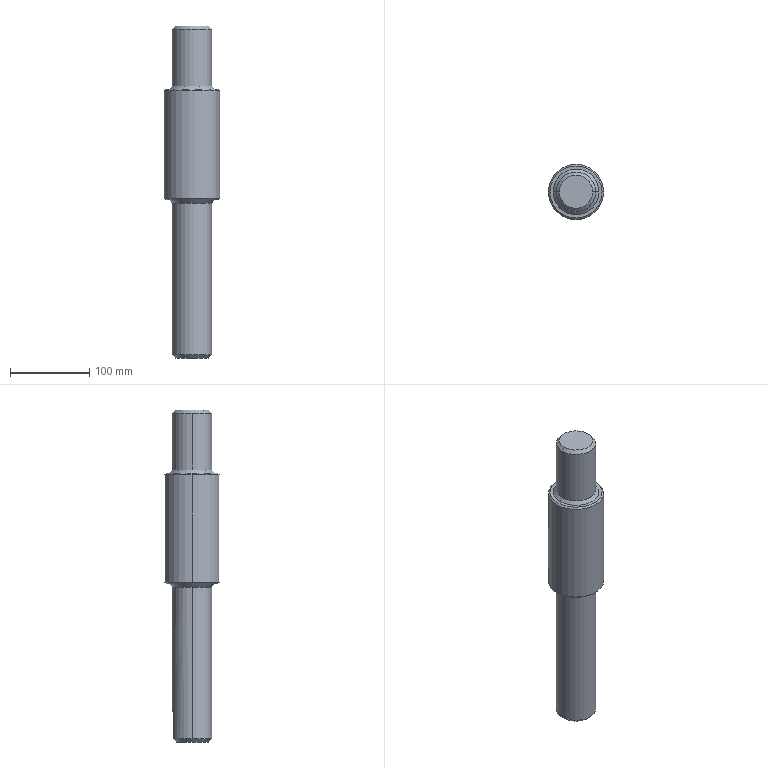Part | SolidWorks | features Chamfer 3, ICE 2, Extrusion 1 | 1 solid | 28 faces | box 70 x 70 x 420 mm | volume 1082180 mm3 | cone 13 | cylinder 8 | plane 7 | commonest cylinder face diameters 50 x4 15 x2 70 x2
STEP:
#1=CARTESIAN_POINT('',(25.,0.,324.));
#2=VERTEX_POINT('',#1);
#3=CARTESIAN_POINT('',(-25.,0.,324.));
#4=VERTEX_POINT('',#3);
#5=CARTESIAN_POINT('',(0.,0.,324.));
#6=DIRECTION('',(0.,0.,1.));
#7=DIRECTION('',(1.,0.,0.));
#8=AXIS2_PLACEMENT_3D('',#5,#6,#7);
#9=CIRCLE('',#8,25.);
#10=EDGE_CURVE('',#2,#4,#9,.T.);
#11=ORIENTED_EDGE('',*,*,#10,.F.);
#12=CARTESIAN_POINT('',(29.,0.,320.));
#13=VERTEX_POINT('',#12);
#14=CARTESIAN_POINT('',(29.,0.,320.));
#15=DIRECTION('',(0.7071,0.,-0.7071));
#16=VECTOR('',#15,1000.);
#17=LINE('',#14,#16);
#18=EDGE_CURVE('',#2,#13,#17,.T.);
#19=ORIENTED_EDGE('',*,*,#18,.T.);
#20=CARTESIAN_POINT('',(-29.,0.,320.));
#21=VERTEX_POINT('',#20);
#22=CARTESIAN_POINT('',(0.,0.,320.));
#23=DIRECTION('',(0.,0.,-1.));
#24=DIRECTION('',(1.,0.,0.));
#25=AXIS2_PLACEMENT_3D('',#22,#23,#24);
#26=CIRCLE('',#25,29.);
#27=EDGE_CURVE('',#21,#13,#26,.T.);
#28=ORIENTED_EDGE('',*,*,#27,.F.);
#29=CARTESIAN_POINT('',(-29.,0.,320.));
#30=DIRECTION('',(-0.7071,0.,-0.7071));
#31=VECTOR('',#30,1000.);
#32=LINE('',#29,#31);
#33=EDGE_CURVE('',#4,#21,#32,.T.);
#34=ORIENTED_EDGE('',*,*,#33,.F.);
#35=EDGE_LOOP('',(#11,#19,#28,#34));
#36=FACE_OUTER_BOUND('',#35,.T.);
#37=CARTESIAN_POINT('',(0.,0.,320.));
#38=DIRECTION('',(0.,0.,-1.));
#39=DIRECTION('',(-1.,0.,0.));
#40=AXIS2_PLACEMENT_3D('',#37,#38,#39);
#41=CONICAL_SURFACE('',#40,29.,0.7854);
#42=ADVANCED_FACE('',(#36),#41,.T.);
#43=CARTESIAN_POINT('',(-25.,0.,176.));
#44=VERTEX_POINT('',#43);
#45=CARTESIAN_POINT('',(25.,0.,176.));
#46=VERTEX_POINT('',#45);
#47=CARTESIAN_POINT('',(0.,0.,176.));
#48=DIRECTION('',(0.,0.,-1.));
#49=DIRECTION('',(1.,0.,0.));
#50=AXIS2_PLACEMENT_3D('',#47,#48,#49);
#51=CIRCLE('',#50,25.);
#52=EDGE_CURVE('',#44,#46,#51,.T.);
#53=ORIENTED_EDGE('',*,*,#52,.F.);
#54=CARTESIAN_POINT('',(-29.,0.,180.));
#55=VERTEX_POINT('',#54);
#56=CARTESIAN_POINT('',(-25.,0.,176.));
#57=DIRECTION('',(-0.7071,0.,0.7071));
#58=VECTOR('',#57,1000.);
#59=LINE('',#56,#58);
#60=EDGE_CURVE('',#44,#55,#59,.T.);
#61=ORIENTED_EDGE('',*,*,#60,.T.);
#62=CARTESIAN_POINT('',(29.,0.,180.));
#63=VERTEX_POINT('',#62);
#64=CARTESIAN_POINT('',(0.,0.,180.));
#65=DIRECTION('',(0.,0.,1.));
#66=DIRECTION('',(1.,0.,0.));
#67=AXIS2_PLACEMENT_3D('',#64,#65,#66);
#68=CIRCLE('',#67,29.);
#69=EDGE_CURVE('',#63,#55,#68,.T.);
#70=ORIENTED_EDGE('',*,*,#69,.F.);
#71=CARTESIAN_POINT('',(25.,0.,176.));
#72=DIRECTION('',(0.7071,0.,0.7071));
#73=VECTOR('',#72,1000.);
#74=LINE('',#71,#73);
#75=EDGE_CURVE('',#46,#63,#74,.T.);
#76=ORIENTED_EDGE('',*,*,#75,.F.);
#77=EDGE_LOOP('',(#53,#61,#70,#76));
#78=FACE_OUTER_BOUND('',#77,.T.);
#79=CARTESIAN_POINT('',(0.,0.,176.));
#80=DIRECTION('',(0.,0.,1.));
#81=DIRECTION('',(1.,0.,0.));
#82=AXIS2_PLACEMENT_3D('',#79,#80,#81);
#83=CONICAL_SURFACE('',#82,25.,0.7854);
#84=ADVANCED_FACE('',(#78),#83,.T.);
#85=CARTESIAN_POINT('',(33.,0.,320.));
#86=VERTEX_POINT('',#85);
#87=CARTESIAN_POINT('',(-33.,0.,320.));
#88=VERTEX_POINT('',#87);
#89=CARTESIAN_POINT('',(0.,0.,320.));
#90=DIRECTION('',(0.,0.,1.));
#91=DIRECTION('',(1.,0.,0.));
#92=AXIS2_PLACEMENT_3D('',#89,#90,#91);
#93=CIRCLE('',#92,33.);
#94=EDGE_CURVE('',#86,#88,#93,.T.);
#95=ORIENTED_EDGE('',*,*,#94,.F.);
#96=CARTESIAN_POINT('',(35.,0.,318.));
#97=VERTEX_POINT('',#96);
#98=CARTESIAN_POINT('',(33.,0.,320.));
#99=DIRECTION('',(0.7071,0.,-0.7071));
#100=VECTOR('',#99,1000.);
#101=LINE('',#98,#100);
#102=EDGE_CURVE('',#86,#97,#101,.T.);
#103=ORIENTED_EDGE('',*,*,#102,.T.);
#104=CARTESIAN_POINT('',(-35.,0.,318.));
#105=VERTEX_POINT('',#104);
#106=CARTESIAN_POINT('',(0.,0.,318.));
#107=DIRECTION('',(0.,0.,-1.));
#108=DIRECTION('',(1.,0.,0.));
#109=AXIS2_PLACEMENT_3D('',#106,#107,#108);
#110=CIRCLE('',#109,35.);
#111=EDGE_CURVE('',#105,#97,#110,.T.);
#112=ORIENTED_EDGE('',*,*,#111,.F.);
#113=CARTESIAN_POINT('',(-33.,0.,320.));
#114=DIRECTION('',(-0.7071,0.,-0.7071));
#115=VECTOR('',#114,1000.);
#116=LINE('',#113,#115);
#117=EDGE_CURVE('',#88,#105,#116,.T.);
#118=ORIENTED_EDGE('',*,*,#117,.F.);
#119=EDGE_LOOP('',(#95,#103,#112,#118));
#120=FACE_OUTER_BOUND('',#119,.T.);
#121=CARTESIAN_POINT('',(0.,0.,320.));
#122=DIRECTION('',(0.,0.,-1.));
#123=DIRECTION('',(-1.,0.,0.));
#124=AXIS2_PLACEMENT_3D('',#121,#122,#123);
#125=CONICAL_SURFACE('',#124,33.,0.7854);
#126=ADVANCED_FACE('',(#120),#125,.T.);
#127=CARTESIAN_POINT('',(-33.,0.,180.));
#128=VERTEX_POINT('',#127);
#129=CARTESIAN_POINT('',(33.,0.,180.));
#130=VERTEX_POINT('',#129);
#131=CARTESIAN_POINT('',(0.,0.,180.));
#132=DIRECTION('',(0.,0.,-1.));
#133=DIRECTION('',(1.,0.,0.));
#134=AXIS2_PLACEMENT_3D('',#131,#132,#133);
#135=CIRCLE('',#134,33.);
#136=EDGE_CURVE('',#128,#130,#135,.T.);
#137=ORIENTED_EDGE('',*,*,#136,.F.);
#138=CARTESIAN_POINT('',(-35.,0.,182.));
#139=VERTEX_POINT('',#138);
#140=CARTESIAN_POINT('',(-35.,0.,182.));
#141=DIRECTION('',(-0.7071,0.,0.7071));
#142=VECTOR('',#141,1000.);
#143=LINE('',#140,#142);
#144=EDGE_CURVE('',#128,#139,#143,.T.);
#145=ORIENTED_EDGE('',*,*,#144,.T.);
#146=CARTESIAN_POINT('',(35.,0.,182.));
#147=VERTEX_POINT('',#146);
#148=CARTESIAN_POINT('',(0.,0.,182.));
#149=DIRECTION('',(0.,0.,1.));
#150=DIRECTION('',(1.,0.,0.));
#151=AXIS2_PLACEMENT_3D('',#148,#149,#150);
#152=CIRCLE('',#151,35.);
#153=EDGE_CURVE('',#147,#139,#152,.T.);
#154=ORIENTED_EDGE('',*,*,#153,.F.);
#155=CARTESIAN_POINT('',(35.,0.,182.));
#156=DIRECTION('',(0.7071,0.,0.7071));
#157=VECTOR('',#156,1000.);
#158=LINE('',#155,#157);
#159=EDGE_CURVE('',#130,#147,#158,.T.);
#160=ORIENTED_EDGE('',*,*,#159,.F.);
#161=EDGE_LOOP('',(#137,#145,#154,#160));
#162=FACE_OUTER_BOUND('',#161,.T.);
#163=CARTESIAN_POINT('',(0.,0.,182.));
#164=DIRECTION('',(0.,0.,1.));
#165=DIRECTION('',(1.,0.,0.));
#166=AXIS2_PLACEMENT_3D('',#163,#164,#165);
#167=CONICAL_SURFACE('',#166,35.,0.7854);
#168=ADVANCED_FACE('',(#162),#167,.T.);
#169=CARTESIAN_POINT('',(-7.5,23.848,-16.));
#170=VERTEX_POINT('',#169);
#171=CARTESIAN_POINT('',(-25.,0.,-16.));
#172=VERTEX_POINT('',#171);
#173=CARTESIAN_POINT('',(0.,0.,-16.));
#174=DIRECTION('',(0.,0.,1.));
#175=DIRECTION('',(1.,0.,0.));
#176=AXIS2_PLACEMENT_3D('',#173,#174,#175);
#177=CIRCLE('',#176,25.);
#178=EDGE_CURVE('',#170,#172,#177,.T.);
#179=ORIENTED_EDGE('',*,*,#178,.T.);
#180=CARTESIAN_POINT('',(-25.,0.,-20.));
#181=DIRECTION('',(0.,0.,1.));
#182=VECTOR('',#181,1000.);
#183=LINE('',#180,#182);
#184=EDGE_CURVE('',#172,#44,#183,.T.);
#185=ORIENTED_EDGE('',*,*,#184,.T.);
#186=ORIENTED_EDGE('',*,*,#52,.T.);
#187=CARTESIAN_POINT('',(25.,0.,-16.));
#188=VERTEX_POINT('',#187);
#189=CARTESIAN_POINT('',(25.,0.,-20.));
#190=DIRECTION('',(0.,0.,1.));
#191=VECTOR('',#190,1000.);
#192=LINE('',#189,#191);
#193=EDGE_CURVE('',#188,#46,#192,.T.);
#194=ORIENTED_EDGE('',*,*,#193,.F.);
#195=CARTESIAN_POINT('',(7.5,23.848,-16.));
#196=VERTEX_POINT('',#195);
#197=CARTESIAN_POINT('',(0.,0.,-16.));
#198=DIRECTION('',(0.,0.,1.));
#199=DIRECTION('',(1.,0.,0.));
#200=AXIS2_PLACEMENT_3D('',#197,#198,#199);
#201=CIRCLE('',#200,25.);
#202=EDGE_CURVE('',#188,#196,#201,.T.);
#203=ORIENTED_EDGE('',*,*,#202,.T.);
#204=CARTESIAN_POINT('',(7.5,23.848,15.));
#205=VERTEX_POINT('',#204);
#206=CARTESIAN_POINT('',(7.5,23.848,-20.));
#207=DIRECTION('',(0.,0.,-1.));
#208=VECTOR('',#207,1000.);
#209=LINE('',#206,#208);
#210=EDGE_CURVE('',#205,#196,#209,.T.);
#211=ORIENTED_EDGE('',*,*,#210,.F.);
#212=CARTESIAN_POINT('',(0.,25.,22.5));
#213=VERTEX_POINT('',#212);
#214=CARTESIAN_POINT('',(0.,25.,22.5));
#215=CARTESIAN_POINT('',(0.492,25.,22.5));
#216=CARTESIAN_POINT('',(0.9918,24.985,22.45));
#217=CARTESIAN_POINT('',(1.955,24.928,22.257));
#218=CARTESIAN_POINT('',(2.424,24.886,22.115));
#219=CARTESIAN_POINT('',(3.107,24.807,21.831));
#220=CARTESIAN_POINT('',(3.331,24.778,21.724));
#221=CARTESIAN_POINT('',(3.762,24.716,21.493));
#222=CARTESIAN_POINT('',(3.971,24.684,21.367));
#223=CARTESIAN_POINT('',(4.375,24.615,21.097));
#224=CARTESIAN_POINT('',(4.571,24.579,20.951));
#225=CARTESIAN_POINT('',(4.948,24.506,20.641));
#226=CARTESIAN_POINT('',(5.131,24.468,20.475));
#227=CARTESIAN_POINT('',(5.65,24.356,19.956));
#228=CARTESIAN_POINT('',(5.958,24.281,19.581));
#229=CARTESIAN_POINT('',(6.501,24.142,18.772));
#230=CARTESIAN_POINT('',(6.736,24.076,18.334));
#231=CARTESIAN_POINT('',(7.112,23.968,17.431));
#232=CARTESIAN_POINT('',(7.255,23.924,16.964));
#233=CARTESIAN_POINT('',(7.401,23.879,16.238));
#234=CARTESIAN_POINT('',(7.438,23.868,15.991));
#235=CARTESIAN_POINT('',(7.488,23.852,15.497));
#236=CARTESIAN_POINT('',(7.5,23.848,15.249));
#237=CARTESIAN_POINT('',(7.5,23.848,15.));
#238=B_SPLINE_CURVE_WITH_KNOTS('',3,(#214,#215,#216,#217,#218,#219,#220,#221,#222,#223,#224,#225,#226,#227,#228,#229,#230,#231,#232,#233,#234,#235,#236,#237),.UNSPECIFIED.,.F.,.F.,(4,2,2,2,2,2,2,2,2,2,2,4),(0.0118,0.01327,0.01474,0.01548,0.01621,0.01695,0.01769,0.01916,0.02063,0.0221,0.02284,0.02358),.UNSPECIFIED.);
#239=EDGE_CURVE('',#213,#205,#238,.T.);
#240=ORIENTED_EDGE('',*,*,#239,.F.);
#241=CARTESIAN_POINT('',(-7.5,23.848,15.));
#242=VERTEX_POINT('',#241);
#243=CARTESIAN_POINT('',(-7.5,23.848,15.));
#244=CARTESIAN_POINT('',(-7.5,23.848,15.499));
#245=CARTESIAN_POINT('',(-7.451,23.864,15.989));
#246=CARTESIAN_POINT('',(-7.306,23.909,16.711));
#247=CARTESIAN_POINT('',(-7.246,23.927,16.949));
#248=CARTESIAN_POINT('',(-7.102,23.97,17.422));
#249=CARTESIAN_POINT('',(-7.018,23.995,17.656));
#250=CARTESIAN_POINT('',(-6.735,24.077,18.336));
#251=CARTESIAN_POINT('',(-6.504,24.141,18.766));
#252=CARTESIAN_POINT('',(-6.096,24.246,19.376));
#253=CARTESIAN_POINT('',(-5.948,24.283,19.574));
#254=CARTESIAN_POINT('',(-5.637,24.357,19.953));
#255=CARTESIAN_POINT('',(-5.473,24.394,20.134));
#256=CARTESIAN_POINT('',(-4.957,24.506,20.649));
#257=CARTESIAN_POINT('',(-4.581,24.58,20.959));
#258=CARTESIAN_POINT('',(-3.761,24.719,21.507));
#259=CARTESIAN_POINT('',(-3.329,24.781,21.738));
#260=CARTESIAN_POINT('',(-2.653,24.86,22.019));
#261=CARTESIAN_POINT('',(-2.423,24.883,22.102));
#262=CARTESIAN_POINT('',(-1.951,24.925,22.246));
#263=CARTESIAN_POINT('',(-1.709,24.943,22.307));
#264=CARTESIAN_POINT('',(-0.9814,24.985,22.452));
#265=CARTESIAN_POINT('',(-0.4926,25.,22.5));
#266=CARTESIAN_POINT('',(0.,25.,22.5));
#267=B_SPLINE_CURVE_WITH_KNOTS('',3,(#243,#244,#245,#246,#247,#248,#249,#250,#251,#252,#253,#254,#255,#256,#257,#258,#259,#260,#261,#262,#263,#264,#265,#266),.UNSPECIFIED.,.F.,.F.,(4,2,2,2,2,2,2,2,2,2,2,4),(0.,0.001474,0.002212,0.002949,0.004423,0.005161,0.005898,0.007372,0.008847,0.009584,0.01032,0.0118),.UNSPECIFIED.);
#268=EDGE_CURVE('',#242,#213,#267,.T.);
#269=ORIENTED_EDGE('',*,*,#268,.F.);
#270=CARTESIAN_POINT('',(-7.5,23.848,-20.));
#271=DIRECTION('',(0.,0.,1.));
#272=VECTOR('',#271,1000.);
#273=LINE('',#270,#272);
#274=EDGE_CURVE('',#170,#242,#273,.T.);
#275=ORIENTED_EDGE('',*,*,#274,.F.);
#276=EDGE_LOOP('',(#179,#185,#186,#194,#203,#211,#240,#269,#275));
#277=FACE_OUTER_BOUND('',#276,.T.);
#278=CARTESIAN_POINT('',(0.,0.,-20.));
#279=DIRECTION('',(0.,0.,1.));
#280=DIRECTION('',(1.,0.,0.));
#281=AXIS2_PLACEMENT_3D('',#278,#279,#280);
#282=CYLINDRICAL_SURFACE('',#281,25.);
#283=ADVANCED_FACE('',(#277),#282,.T.);
#284=CARTESIAN_POINT('',(-21.,0.,-20.));
#285=VERTEX_POINT('',#284);
#286=CARTESIAN_POINT('',(-7.5,19.615,-20.));
#287=VERTEX_POINT('',#286);
#288=CARTESIAN_POINT('',(0.,0.,-20.));
#289=DIRECTION('',(0.,0.,-1.));
#290=DIRECTION('',(1.,0.,0.));
#291=AXIS2_PLACEMENT_3D('',#288,#289,#290);
#292=CIRCLE('',#291,21.);
#293=EDGE_CURVE('',#285,#287,#292,.T.);
#294=ORIENTED_EDGE('',*,*,#293,.F.);
#295=CARTESIAN_POINT('',(-25.,0.,-16.));
#296=DIRECTION('',(-0.7071,0.,0.7071));
#297=VECTOR('',#296,1000.);
#298=LINE('',#295,#297);
#299=EDGE_CURVE('',#285,#172,#298,.T.);
#300=ORIENTED_EDGE('',*,*,#299,.T.);
#301=ORIENTED_EDGE('',*,*,#178,.F.);
#302=CARTESIAN_POINT('',(-7.5,19.615,-20.));
#303=CARTESIAN_POINT('',(-7.5,21.034,-18.675));
#304=CARTESIAN_POINT('',(-7.5,22.444,-17.34));
#305=CARTESIAN_POINT('',(-7.5,23.848,-16.));
#306=B_SPLINE_CURVE_WITH_KNOTS('',3,(#302,#303,#304,#305),.UNSPECIFIED.,.F.,.F.,(4,4),(0.02102,0.02682),.UNSPECIFIED.);
#307=EDGE_CURVE('',#287,#170,#306,.T.);
#308=ORIENTED_EDGE('',*,*,#307,.F.);
#309=EDGE_LOOP('',(#294,#300,#301,#308));
#310=FACE_OUTER_BOUND('',#309,.T.);
#311=CARTESIAN_POINT('',(0.,0.,-16.));
#312=DIRECTION('',(0.,0.,1.));
#313=DIRECTION('',(1.,0.,0.));
#314=AXIS2_PLACEMENT_3D('',#311,#312,#313);
#315=CONICAL_SURFACE('',#314,25.,0.7854);
#316=ADVANCED_FACE('',(#310),#315,.T.);
#317=ORIENTED_EDGE('',*,*,#299,.F.);
#318=CARTESIAN_POINT('',(21.,0.,-20.));
#319=VERTEX_POINT('',#318);
#320=CARTESIAN_POINT('',(0.,0.,-20.));
#321=DIRECTION('',(0.,0.,-1.));
#322=DIRECTION('',(1.,0.,0.));
#323=AXIS2_PLACEMENT_3D('',#320,#321,#322);
#324=CIRCLE('',#323,21.);
#325=EDGE_CURVE('',#319,#285,#324,.T.);
#326=ORIENTED_EDGE('',*,*,#325,.F.);
#327=CARTESIAN_POINT('',(25.,0.,-16.));
#328=DIRECTION('',(0.7071,0.,0.7071));
#329=VECTOR('',#328,1000.);
#330=LINE('',#327,#329);
#331=EDGE_CURVE('',#319,#188,#330,.T.);
#332=ORIENTED_EDGE('',*,*,#331,.T.);
#333=CARTESIAN_POINT('',(0.,0.,-16.));
#334=DIRECTION('',(0.,0.,1.));
#335=DIRECTION('',(1.,0.,0.));
#336=AXIS2_PLACEMENT_3D('',#333,#334,#335);
#337=CIRCLE('',#336,25.);
#338=EDGE_CURVE('',#172,#188,#337,.T.);
#339=ORIENTED_EDGE('',*,*,#338,.F.);
#340=EDGE_LOOP('',(#317,#326,#332,#339));
#341=FACE_OUTER_BOUND('',#340,.T.);
#342=CARTESIAN_POINT('',(0.,0.,-16.));
#343=DIRECTION('',(0.,0.,1.));
#344=DIRECTION('',(1.,0.,0.));
#345=AXIS2_PLACEMENT_3D('',#342,#343,#344);
#346=CONICAL_SURFACE('',#345,25.,0.7854);
#347=ADVANCED_FACE('',(#341),#346,.T.);
#348=CARTESIAN_POINT('',(0.,15.,22.5));
#349=VERTEX_POINT('',#348);
#350=CARTESIAN_POINT('',(7.5,15.,15.));
#351=VERTEX_POINT('',#350);
#352=CARTESIAN_POINT('',(0.,15.,15.));
#353=DIRECTION('',(0.,1.,0.));
#354=DIRECTION('',(0.,0.,1.));
#355=AXIS2_PLACEMENT_3D('',#352,#353,#354);
#356=CIRCLE('',#355,7.5);
#357=EDGE_CURVE('',#349,#351,#356,.T.);
#358=ORIENTED_EDGE('',*,*,#357,.F.);
#359=CARTESIAN_POINT('',(0.,15.,22.5));
#360=DIRECTION('',(0.,1.,0.));
#361=VECTOR('',#360,1000.);
#362=LINE('',#359,#361);
#363=EDGE_CURVE('',#349,#213,#362,.T.);
#364=ORIENTED_EDGE('',*,*,#363,.T.);
#365=ORIENTED_EDGE('',*,*,#239,.T.);
#366=CARTESIAN_POINT('',(7.5,15.,15.));
#367=DIRECTION('',(0.,1.,0.));
#368=VECTOR('',#367,1000.);
#369=LINE('',#366,#368);
#370=EDGE_CURVE('',#351,#205,#369,.T.);
#371=ORIENTED_EDGE('',*,*,#370,.F.);
#372=EDGE_LOOP('',(#358,#364,#365,#371));
#373=FACE_OUTER_BOUND('',#372,.T.);
#374=CARTESIAN_POINT('',(0.,15.,15.));
#375=DIRECTION('',(0.,1.,0.));
#376=DIRECTION('',(0.,0.,1.));
#377=AXIS2_PLACEMENT_3D('',#374,#375,#376);
#378=CYLINDRICAL_SURFACE('',#377,7.5);
#379=ADVANCED_FACE('',(#373),#378,.F.);
#380=ORIENTED_EDGE('',*,*,#111,.T.);
#381=CARTESIAN_POINT('',(35.,0.,320.));
#382=DIRECTION('',(0.,0.,-1.));
#383=VECTOR('',#382,1000.);
#384=LINE('',#381,#383);
#385=EDGE_CURVE('',#97,#147,#384,.T.);
#386=ORIENTED_EDGE('',*,*,#385,.T.);
#387=ORIENTED_EDGE('',*,*,#153,.T.);
#388=CARTESIAN_POINT('',(-35.,0.,320.));
#389=DIRECTION('',(0.,0.,-1.));
#390=VECTOR('',#389,1000.);
#391=LINE('',#388,#390);
#392=EDGE_CURVE('',#105,#139,#391,.T.);
#393=ORIENTED_EDGE('',*,*,#392,.F.);
#394=EDGE_LOOP('',(#380,#386,#387,#393));
#395=FACE_OUTER_BOUND('',#394,.T.);
#396=CARTESIAN_POINT('',(0.,0.,320.));
#397=DIRECTION('',(0.,0.,-1.));
#398=DIRECTION('',(-1.,0.,0.));
#399=AXIS2_PLACEMENT_3D('',#396,#397,#398);
#400=CYLINDRICAL_SURFACE('',#399,35.);
#401=ADVANCED_FACE('',(#395),#400,.T.);
#402=CARTESIAN_POINT('',(21.,0.,400.));
#403=VERTEX_POINT('',#402);
#404=CARTESIAN_POINT('',(-21.,0.,400.));
#405=VERTEX_POINT('',#404);
#406=CARTESIAN_POINT('',(0.,0.,400.));
#407=DIRECTION('',(0.,0.,1.));
#408=DIRECTION('',(1.,0.,0.));
#409=AXIS2_PLACEMENT_3D('',#406,#407,#408);
#410=CIRCLE('',#409,21.);
#411=EDGE_CURVE('',#403,#405,#410,.T.);
#412=ORIENTED_EDGE('',*,*,#411,.F.);
#413=CARTESIAN_POINT('',(25.,0.,396.));
#414=VERTEX_POINT('',#413);
#415=CARTESIAN_POINT('',(21.,0.,400.));
#416=DIRECTION('',(0.7071,0.,-0.7071));
#417=VECTOR('',#416,1000.);
#418=LINE('',#415,#417);
#419=EDGE_CURVE('',#403,#414,#418,.T.);
#420=ORIENTED_EDGE('',*,*,#419,.T.);
#421=CARTESIAN_POINT('',(-25.,0.,396.));
#422=VERTEX_POINT('',#421);
#423=CARTESIAN_POINT('',(0.,0.,396.));
#424=DIRECTION('',(0.,0.,-1.));
#425=DIRECTION('',(1.,0.,0.));
#426=AXIS2_PLACEMENT_3D('',#423,#424,#425);
#427=CIRCLE('',#426,25.);
#428=EDGE_CURVE('',#422,#414,#427,.T.);
#429=ORIENTED_EDGE('',*,*,#428,.F.);
#430=CARTESIAN_POINT('',(-21.,0.,400.));
#431=DIRECTION('',(-0.7071,0.,-0.7071));
#432=VECTOR('',#431,1000.);
#433=LINE('',#430,#432);
#434=EDGE_CURVE('',#405,#422,#433,.T.);
#435=ORIENTED_EDGE('',*,*,#434,.F.);
#436=EDGE_LOOP('',(#412,#420,#429,#435));
#437=FACE_OUTER_BOUND('',#436,.T.);
#438=CARTESIAN_POINT('',(0.,0.,400.));
#439=DIRECTION('',(0.,0.,-1.));
#440=DIRECTION('',(-1.,0.,0.));
#441=AXIS2_PLACEMENT_3D('',#438,#439,#440);
#442=CONICAL_SURFACE('',#441,21.,0.7854);
#443=ADVANCED_FACE('',(#437),#442,.T.);
#444=ORIENTED_EDGE('',*,*,#10,.T.);
#445=CARTESIAN_POINT('',(-25.,0.,-20.));
#446=DIRECTION('',(0.,0.,1.));
#447=VECTOR('',#446,1000.);
#448=LINE('',#445,#447);
#449=EDGE_CURVE('',#4,#422,#448,.T.);
#450=ORIENTED_EDGE('',*,*,#449,.T.);
#451=ORIENTED_EDGE('',*,*,#428,.T.);
#452=CARTESIAN_POINT('',(25.,0.,-20.));
#453=DIRECTION('',(0.,0.,1.));
#454=VECTOR('',#453,1000.);
#455=LINE('',#452,#454);
#456=EDGE_CURVE('',#2,#414,#455,.T.);
#457=ORIENTED_EDGE('',*,*,#456,.F.);
#458=EDGE_LOOP('',(#444,#450,#451,#457));
#459=FACE_OUTER_BOUND('',#458,.T.);
#460=CARTESIAN_POINT('',(0.,0.,-20.));
#461=DIRECTION('',(0.,0.,1.));
#462=DIRECTION('',(1.,0.,0.));
#463=AXIS2_PLACEMENT_3D('',#460,#461,#462);
#464=CYLINDRICAL_SURFACE('',#463,25.);
#465=ADVANCED_FACE('',(#459),#464,.T.);
#466=ORIENTED_EDGE('',*,*,#449,.F.);
#467=CARTESIAN_POINT('',(0.,0.,324.));
#468=DIRECTION('',(0.,0.,1.));
#469=DIRECTION('',(1.,0.,0.));
#470=AXIS2_PLACEMENT_3D('',#467,#468,#469);
#471=CIRCLE('',#470,25.);
#472=EDGE_CURVE('',#4,#2,#471,.T.);
#473=ORIENTED_EDGE('',*,*,#472,.T.);
#474=ORIENTED_EDGE('',*,*,#456,.T.);
#475=CARTESIAN_POINT('',(0.,0.,396.));
#476=DIRECTION('',(0.,0.,-1.));
#477=DIRECTION('',(1.,0.,0.));
#478=AXIS2_PLACEMENT_3D('',#475,#476,#477);
#479=CIRCLE('',#478,25.);
#480=EDGE_CURVE('',#414,#422,#479,.T.);
#481=ORIENTED_EDGE('',*,*,#480,.T.);
#482=EDGE_LOOP('',(#466,#473,#474,#481));
#483=FACE_OUTER_BOUND('',#482,.T.);
#484=CARTESIAN_POINT('',(0.,0.,-20.));
#485=DIRECTION('',(0.,0.,1.));
#486=DIRECTION('',(1.,0.,0.));
#487=AXIS2_PLACEMENT_3D('',#484,#485,#486);
#488=CYLINDRICAL_SURFACE('',#487,25.);
#489=ADVANCED_FACE('',(#483),#488,.T.);
#490=CARTESIAN_POINT('',(0.,0.,400.));
#491=DIRECTION('',(0.,0.,1.));
#492=DIRECTION('',(1.,0.,0.));
#493=AXIS2_PLACEMENT_3D('',#490,#491,#492);
#494=CIRCLE('',#493,21.);
#495=EDGE_CURVE('',#405,#403,#494,.T.);
#496=ORIENTED_EDGE('',*,*,#495,.T.);
#497=ORIENTED_EDGE('',*,*,#411,.T.);
#498=EDGE_LOOP('',(#496,#497));
#499=FACE_OUTER_BOUND('',#498,.T.);
#500=CARTESIAN_POINT('',(0.,0.,400.));
#501=DIRECTION('',(0.,0.,1.));
#502=DIRECTION('',(1.,0.,0.));
#503=AXIS2_PLACEMENT_3D('',#500,#501,#502);
#504=PLANE('',#503);
#505=ADVANCED_FACE('',(#499),#504,.T.);
#506=ORIENTED_EDGE('',*,*,#419,.F.);
#507=ORIENTED_EDGE('',*,*,#495,.F.);
#508=ORIENTED_EDGE('',*,*,#434,.T.);
#509=ORIENTED_EDGE('',*,*,#480,.F.);
#510=EDGE_LOOP('',(#506,#507,#508,#509));
#511=FACE_OUTER_BOUND('',#510,.T.);
#512=CARTESIAN_POINT('',(0.,0.,400.));
#513=DIRECTION('',(0.,0.,-1.));
#514=DIRECTION('',(-1.,0.,0.));
#515=AXIS2_PLACEMENT_3D('',#512,#513,#514);
#516=CONICAL_SURFACE('',#515,21.,0.7854);
#517=ADVANCED_FACE('',(#511),#516,.T.);
#518=ORIENTED_EDGE('',*,*,#385,.F.);
#519=CARTESIAN_POINT('',(0.,0.,318.));
#520=DIRECTION('',(0.,0.,-1.));
#521=DIRECTION('',(1.,0.,0.));
#522=AXIS2_PLACEMENT_3D('',#519,#520,#521);
#523=CIRCLE('',#522,35.);
#524=EDGE_CURVE('',#97,#105,#523,.T.);
#525=ORIENTED_EDGE('',*,*,#524,.T.);
#526=ORIENTED_EDGE('',*,*,#392,.T.);
#527=CARTESIAN_POINT('',(0.,0.,182.));
#528=DIRECTION('',(0.,0.,1.));
#529=DIRECTION('',(1.,0.,0.));
#530=AXIS2_PLACEMENT_3D('',#527,#528,#529);
#531=CIRCLE('',#530,35.);
#532=EDGE_CURVE('',#139,#147,#531,.T.);
#533=ORIENTED_EDGE('',*,*,#532,.T.);
#534=EDGE_LOOP('',(#518,#525,#526,#533));
#535=FACE_OUTER_BOUND('',#534,.T.);
#536=CARTESIAN_POINT('',(0.,0.,320.));
#537=DIRECTION('',(0.,0.,-1.));
#538=DIRECTION('',(-1.,0.,0.));
#539=AXIS2_PLACEMENT_3D('',#536,#537,#538);
#540=CYLINDRICAL_SURFACE('',#539,35.);
#541=ADVANCED_FACE('',(#535),#540,.T.);
#542=ORIENTED_EDGE('',*,*,#27,.T.);
#543=CARTESIAN_POINT('',(0.,0.,320.));
#544=DIRECTION('',(0.,0.,-1.));
#545=DIRECTION('',(1.,0.,0.));
#546=AXIS2_PLACEMENT_3D('',#543,#544,#545);
#547=CIRCLE('',#546,29.);
#548=EDGE_CURVE('',#13,#21,#547,.T.);
#549=ORIENTED_EDGE('',*,*,#548,.T.);
#550=EDGE_LOOP('',(#542,#549));
#551=FACE_BOUND('',#550,.T.);
#552=CARTESIAN_POINT('',(0.,0.,320.));
#553=DIRECTION('',(0.,0.,1.));
#554=DIRECTION('',(1.,0.,0.));
#555=AXIS2_PLACEMENT_3D('',#552,#553,#554);
#556=CIRCLE('',#555,33.);
#557=EDGE_CURVE('',#88,#86,#556,.T.);
#558=ORIENTED_EDGE('',*,*,#557,.T.);
#559=ORIENTED_EDGE('',*,*,#94,.T.);
#560=EDGE_LOOP('',(#558,#559));
#561=FACE_OUTER_BOUND('',#560,.T.);
#562=CARTESIAN_POINT('',(0.,0.,320.));
#563=DIRECTION('',(0.,0.,1.));
#564=DIRECTION('',(1.,0.,0.));
#565=AXIS2_PLACEMENT_3D('',#562,#563,#564);
#566=PLANE('',#565);
#567=ADVANCED_FACE('',(#551,#561),#566,.T.);
#568=ORIENTED_EDGE('',*,*,#69,.T.);
#569=CARTESIAN_POINT('',(0.,0.,180.));
#570=DIRECTION('',(0.,0.,1.));
#571=DIRECTION('',(1.,0.,0.));
#572=AXIS2_PLACEMENT_3D('',#569,#570,#571);
#573=CIRCLE('',#572,29.);
#574=EDGE_CURVE('',#55,#63,#573,.T.);
#575=ORIENTED_EDGE('',*,*,#574,.T.);
#576=EDGE_LOOP('',(#568,#575));
#577=FACE_BOUND('',#576,.T.);
#578=CARTESIAN_POINT('',(0.,0.,180.));
#579=DIRECTION('',(0.,0.,-1.));
#580=DIRECTION('',(1.,0.,0.));
#581=AXIS2_PLACEMENT_3D('',#578,#579,#580);
#582=CIRCLE('',#581,33.);
#583=EDGE_CURVE('',#130,#128,#582,.T.);
#584=ORIENTED_EDGE('',*,*,#583,.T.);
#585=ORIENTED_EDGE('',*,*,#136,.T.);
#586=EDGE_LOOP('',(#584,#585));
#587=FACE_OUTER_BOUND('',#586,.T.);
#588=CARTESIAN_POINT('',(0.,0.,180.));
#589=DIRECTION('',(0.,0.,1.));
#590=DIRECTION('',(1.,0.,0.));
#591=AXIS2_PLACEMENT_3D('',#588,#589,#590);
#592=PLANE('',#591);
#593=ADVANCED_FACE('',(#577,#587),#592,.F.);
#594=CARTESIAN_POINT('',(7.5,19.615,-20.));
#595=VERTEX_POINT('',#594);
#596=CARTESIAN_POINT('',(0.,0.,-20.));
#597=DIRECTION('',(0.,0.,-1.));
#598=DIRECTION('',(1.,0.,0.));
#599=AXIS2_PLACEMENT_3D('',#596,#597,#598);
#600=CIRCLE('',#599,21.);
#601=EDGE_CURVE('',#595,#319,#600,.T.);
#602=ORIENTED_EDGE('',*,*,#601,.T.);
#603=ORIENTED_EDGE('',*,*,#325,.T.);
#604=ORIENTED_EDGE('',*,*,#293,.T.);
#605=CARTESIAN_POINT('',(-7.5,15.,-20.));
#606=VERTEX_POINT('',#605);
#607=CARTESIAN_POINT('',(-7.5,0.,-20.));
#608=DIRECTION('',(0.,-1.,0.));
#609=VECTOR('',#608,1000.);
#610=LINE('',#607,#609);
#611=EDGE_CURVE('',#287,#606,#610,.T.);
#612=ORIENTED_EDGE('',*,*,#611,.T.);
#613=CARTESIAN_POINT('',(7.5,15.,-20.));
#614=VERTEX_POINT('',#613);
#615=CARTESIAN_POINT('',(0.,15.,-20.));
#616=DIRECTION('',(-1.,0.,0.));
#617=VECTOR('',#616,1000.);
#618=LINE('',#615,#617);
#619=EDGE_CURVE('',#614,#606,#618,.T.);
#620=ORIENTED_EDGE('',*,*,#619,.F.);
#621=CARTESIAN_POINT('',(7.5,0.,-20.));
#622=DIRECTION('',(0.,1.,0.));
#623=VECTOR('',#622,1000.);
#624=LINE('',#621,#623);
#625=EDGE_CURVE('',#614,#595,#624,.T.);
#626=ORIENTED_EDGE('',*,*,#625,.T.);
#627=EDGE_LOOP('',(#602,#603,#604,#612,#620,#626));
#628=FACE_OUTER_BOUND('',#627,.T.);
#629=CARTESIAN_POINT('',(0.,0.,-20.));
#630=DIRECTION('',(0.,0.,1.));
#631=DIRECTION('',(1.,0.,0.));
#632=AXIS2_PLACEMENT_3D('',#629,#630,#631);
#633=PLANE('',#632);
#634=ADVANCED_FACE('',(#628),#633,.F.);
#635=ORIENTED_EDGE('',*,*,#619,.T.);
#636=CARTESIAN_POINT('',(-7.5,15.,15.));
#637=VERTEX_POINT('',#636);
#638=CARTESIAN_POINT('',(-7.5,15.,15.));
#639=DIRECTION('',(0.,0.,1.));
#640=VECTOR('',#639,1000.);
#641=LINE('',#638,#640);
#642=EDGE_CURVE('',#606,#637,#641,.T.);
#643=ORIENTED_EDGE('',*,*,#642,.T.);
#644=CARTESIAN_POINT('',(0.,15.,15.));
#645=DIRECTION('',(0.,1.,0.));
#646=DIRECTION('',(0.,0.,1.));
#647=AXIS2_PLACEMENT_3D('',#644,#645,#646);
#648=CIRCLE('',#647,7.5);
#649=EDGE_CURVE('',#637,#349,#648,.T.);
#650=ORIENTED_EDGE('',*,*,#649,.T.);
#651=ORIENTED_EDGE('',*,*,#357,.T.);
#652=CARTESIAN_POINT('',(7.5,15.,15.));
#653=DIRECTION('',(0.,0.,-1.));
#654=VECTOR('',#653,1000.);
#655=LINE('',#652,#654);
#656=EDGE_CURVE('',#351,#614,#655,.T.);
#657=ORIENTED_EDGE('',*,*,#656,.T.);
#658=EDGE_LOOP('',(#635,#643,#650,#651,#657));
#659=FACE_OUTER_BOUND('',#658,.T.);
#660=CARTESIAN_POINT('',(0.,15.,15.));
#661=DIRECTION('',(0.,1.,0.));
#662=DIRECTION('',(0.,0.,1.));
#663=AXIS2_PLACEMENT_3D('',#660,#661,#662);
#664=PLANE('',#663);
#665=ADVANCED_FACE('',(#659),#664,.T.);
#666=ORIENTED_EDGE('',*,*,#363,.F.);
#667=ORIENTED_EDGE('',*,*,#649,.F.);
#668=CARTESIAN_POINT('',(-7.5,15.,15.));
#669=DIRECTION('',(0.,1.,0.));
#670=VECTOR('',#669,1000.);
#671=LINE('',#668,#670);
#672=EDGE_CURVE('',#637,#242,#671,.T.);
#673=ORIENTED_EDGE('',*,*,#672,.T.);
#674=ORIENTED_EDGE('',*,*,#268,.T.);
#675=EDGE_LOOP('',(#666,#667,#673,#674));
#676=FACE_OUTER_BOUND('',#675,.T.);
#677=CARTESIAN_POINT('',(0.,15.,15.));
#678=DIRECTION('',(0.,1.,0.));
#679=DIRECTION('',(0.,0.,1.));
#680=AXIS2_PLACEMENT_3D('',#677,#678,#679);
#681=CYLINDRICAL_SURFACE('',#680,7.5);
#682=ADVANCED_FACE('',(#676),#681,.F.);
#683=ORIENTED_EDGE('',*,*,#210,.T.);
#684=CARTESIAN_POINT('',(7.5,23.848,-16.));
#685=CARTESIAN_POINT('',(7.5,22.444,-17.34));
#686=CARTESIAN_POINT('',(7.5,21.034,-18.675));
#687=CARTESIAN_POINT('',(7.5,19.615,-20.));
#688=B_SPLINE_CURVE_WITH_KNOTS('',3,(#684,#685,#686,#687),.UNSPECIFIED.,.F.,.F.,(4,4),(0.01654,0.02236),.UNSPECIFIED.);
#689=EDGE_CURVE('',#196,#595,#688,.T.);
#690=ORIENTED_EDGE('',*,*,#689,.T.);
#691=ORIENTED_EDGE('',*,*,#625,.F.);
#692=ORIENTED_EDGE('',*,*,#656,.F.);
#693=ORIENTED_EDGE('',*,*,#370,.T.);
#694=EDGE_LOOP('',(#683,#690,#691,#692,#693));
#695=FACE_OUTER_BOUND('',#694,.T.);
#696=CARTESIAN_POINT('',(7.5,15.,15.));
#697=DIRECTION('',(1.,0.,0.));
#698=DIRECTION('',(0.,0.,-1.));
#699=AXIS2_PLACEMENT_3D('',#696,#697,#698);
#700=PLANE('',#699);
#701=ADVANCED_FACE('',(#695),#700,.F.);
#702=ORIENTED_EDGE('',*,*,#331,.F.);
#703=ORIENTED_EDGE('',*,*,#601,.F.);
#704=ORIENTED_EDGE('',*,*,#689,.F.);
#705=ORIENTED_EDGE('',*,*,#202,.F.);
#706=EDGE_LOOP('',(#702,#703,#704,#705));
#707=FACE_OUTER_BOUND('',#706,.T.);
#708=CARTESIAN_POINT('',(0.,0.,-16.));
#709=DIRECTION('',(0.,0.,1.));
#710=DIRECTION('',(1.,0.,0.));
#711=AXIS2_PLACEMENT_3D('',#708,#709,#710);
#712=CONICAL_SURFACE('',#711,25.,0.7854);
#713=ADVANCED_FACE('',(#707),#712,.T.);
#714=ORIENTED_EDGE('',*,*,#274,.T.);
#715=ORIENTED_EDGE('',*,*,#672,.F.);
#716=ORIENTED_EDGE('',*,*,#642,.F.);
#717=ORIENTED_EDGE('',*,*,#611,.F.);
#718=ORIENTED_EDGE('',*,*,#307,.T.);
#719=EDGE_LOOP('',(#714,#715,#716,#717,#718));
#720=FACE_OUTER_BOUND('',#719,.T.);
#721=CARTESIAN_POINT('',(-7.5,15.,15.));
#722=DIRECTION('',(-1.,0.,0.));
#723=DIRECTION('',(0.,0.,1.));
#724=AXIS2_PLACEMENT_3D('',#721,#722,#723);
#725=PLANE('',#724);
#726=ADVANCED_FACE('',(#720),#725,.F.);
#727=ORIENTED_EDGE('',*,*,#184,.F.);
#728=ORIENTED_EDGE('',*,*,#338,.T.);
#729=ORIENTED_EDGE('',*,*,#193,.T.);
#730=CARTESIAN_POINT('',(0.,0.,176.));
#731=DIRECTION('',(0.,0.,-1.));
#732=DIRECTION('',(1.,0.,0.));
#733=AXIS2_PLACEMENT_3D('',#730,#731,#732);
#734=CIRCLE('',#733,25.);
#735=EDGE_CURVE('',#46,#44,#734,.T.);
#736=ORIENTED_EDGE('',*,*,#735,.T.);
#737=EDGE_LOOP('',(#727,#728,#729,#736));
#738=FACE_OUTER_BOUND('',#737,.T.);
#739=CARTESIAN_POINT('',(0.,0.,-20.));
#740=DIRECTION('',(0.,0.,1.));
#741=DIRECTION('',(1.,0.,0.));
#742=AXIS2_PLACEMENT_3D('',#739,#740,#741);
#743=CYLINDRICAL_SURFACE('',#742,25.);
#744=ADVANCED_FACE('',(#738),#743,.T.);
#745=ORIENTED_EDGE('',*,*,#144,.F.);
#746=ORIENTED_EDGE('',*,*,#583,.F.);
#747=ORIENTED_EDGE('',*,*,#159,.T.);
#748=ORIENTED_EDGE('',*,*,#532,.F.);
#749=EDGE_LOOP('',(#745,#746,#747,#748));
#750=FACE_OUTER_BOUND('',#749,.T.);
#751=CARTESIAN_POINT('',(0.,0.,182.));
#752=DIRECTION('',(0.,0.,1.));
#753=DIRECTION('',(1.,0.,0.));
#754=AXIS2_PLACEMENT_3D('',#751,#752,#753);
#755=CONICAL_SURFACE('',#754,35.,0.7854);
#756=ADVANCED_FACE('',(#750),#755,.T.);
#757=ORIENTED_EDGE('',*,*,#102,.F.);
#758=ORIENTED_EDGE('',*,*,#557,.F.);
#759=ORIENTED_EDGE('',*,*,#117,.T.);
#760=ORIENTED_EDGE('',*,*,#524,.F.);
#761=EDGE_LOOP('',(#757,#758,#759,#760));
#762=FACE_OUTER_BOUND('',#761,.T.);
#763=CARTESIAN_POINT('',(0.,0.,320.));
#764=DIRECTION('',(0.,0.,-1.));
#765=DIRECTION('',(-1.,0.,0.));
#766=AXIS2_PLACEMENT_3D('',#763,#764,#765);
#767=CONICAL_SURFACE('',#766,33.,0.7854);
#768=ADVANCED_FACE('',(#762),#767,.T.);
#769=ORIENTED_EDGE('',*,*,#60,.F.);
#770=ORIENTED_EDGE('',*,*,#735,.F.);
#771=ORIENTED_EDGE('',*,*,#75,.T.);
#772=ORIENTED_EDGE('',*,*,#574,.F.);
#773=EDGE_LOOP('',(#769,#770,#771,#772));
#774=FACE_OUTER_BOUND('',#773,.T.);
#775=CARTESIAN_POINT('',(0.,0.,176.));
#776=DIRECTION('',(0.,0.,1.));
#777=DIRECTION('',(1.,0.,0.));
#778=AXIS2_PLACEMENT_3D('',#775,#776,#777);
#779=CONICAL_SURFACE('',#778,25.,0.7854);
#780=ADVANCED_FACE('',(#774),#779,.T.);
#781=ORIENTED_EDGE('',*,*,#18,.F.);
#782=ORIENTED_EDGE('',*,*,#472,.F.);
#783=ORIENTED_EDGE('',*,*,#33,.T.);
#784=ORIENTED_EDGE('',*,*,#548,.F.);
#785=EDGE_LOOP('',(#781,#782,#783,#784));
#786=FACE_OUTER_BOUND('',#785,.T.);
#787=CARTESIAN_POINT('',(0.,0.,320.));
#788=DIRECTION('',(0.,0.,-1.));
#789=DIRECTION('',(-1.,0.,0.));
#790=AXIS2_PLACEMENT_3D('',#787,#788,#789);
#791=CONICAL_SURFACE('',#790,29.,0.7854);
#792=ADVANCED_FACE('',(#786),#791,.T.);
#793=CLOSED_SHELL('',(#42,#84,#126,#168,#283,#316,#347,#379,#401,#443,#465,#489,#505,#517,#541,#567,#593,#634,#665,#682,#701,#713,#726,#744,#756,#768,#780,#792));
#794=MANIFOLD_SOLID_BREP('',#793);
#795=CARTESIAN_POINT('',(0.,0.,0.));
#796=DIRECTION('',(0.,0.,1.));
#797=DIRECTION('',(1.,0.,0.));
#798=AXIS2_PLACEMENT_3D('',#795,#796,#797);
#799=(LENGTH_UNIT()NAMED_UNIT(*)SI_UNIT(.MILLI.,.METRE.));
#800=UNCERTAINTY_MEASURE_WITH_UNIT(LENGTH_MEASURE(0.00001),#799,'','');
#801=(NAMED_UNIT(*)PLANE_ANGLE_UNIT()SI_UNIT($,.RADIAN.));
#802=(NAMED_UNIT(*)SI_UNIT($,.STERADIAN.)SOLID_ANGLE_UNIT());
#803=(GEOMETRIC_REPRESENTATION_CONTEXT(3)GLOBAL_UNCERTAINTY_ASSIGNED_CONTEXT((#800))GLOBAL_UNIT_ASSIGNED_CONTEXT((#799,#801,#802))REPRESENTATION_CONTEXT('',''));
#804=ADVANCED_BREP_SHAPE_REPRESENTATION('',(#794,#798),#803);